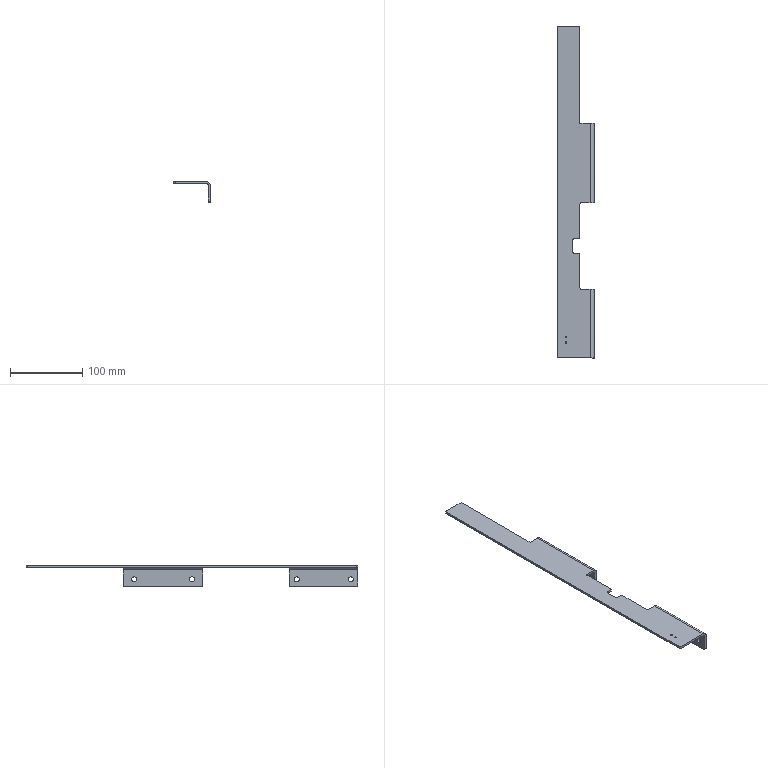Part | NX | features 5003_234_Bracket 2 | 1 solid | 39 faces | box 51 x 460 x 29 mm | volume 68788 mm3 | plane 20 | cylinder 19 | commonest cylinder face diameters 4 x9 7 x4 2.5 x2 6 x2 12 x2
STEP:
#1=CARTESIAN_POINT('',(-224.475,-262.,-64.));
#2=VERTEX_POINT('',#1);
#3=CARTESIAN_POINT('',(-227.475,-262.,-61.));
#4=VERTEX_POINT('',#3);
#5=CARTESIAN_POINT('',(-227.475,-262.,-64.));
#6=DIRECTION('',(0.,1.,0.));
#7=DIRECTION('',(-1.,0.,0.));
#8=AXIS2_PLACEMENT_3D('',#5,#6,#7);
#9=CIRCLE('',#8,3.);
#10=EDGE_CURVE('',#2,#4,#9,.F.);
#11=ORIENTED_EDGE('',*,*,#10,.T.);
#12=CARTESIAN_POINT('',(-227.475,-152.,-61.));
#13=VERTEX_POINT('',#12);
#14=CARTESIAN_POINT('',(-227.475,-477.,-61.));
#15=DIRECTION('',(0.,1.,0.));
#16=VECTOR('',#15,1000.);
#17=LINE('',#14,#16);
#18=EDGE_CURVE('',#4,#13,#17,.T.);
#19=ORIENTED_EDGE('',*,*,#18,.T.);
#20=CARTESIAN_POINT('',(-224.475,-152.,-64.));
#21=VERTEX_POINT('',#20);
#22=CARTESIAN_POINT('',(-227.475,-152.,-64.));
#23=DIRECTION('',(0.,-1.,0.));
#24=DIRECTION('',(1.,0.,0.));
#25=AXIS2_PLACEMENT_3D('',#22,#23,#24);
#26=CIRCLE('',#25,3.);
#27=EDGE_CURVE('',#13,#21,#26,.F.);
#28=ORIENTED_EDGE('',*,*,#27,.T.);
#29=CARTESIAN_POINT('',(-224.475,-477.,-64.));
#30=DIRECTION('',(0.,1.,0.));
#31=VECTOR('',#30,1000.);
#32=LINE('',#29,#31);
#33=EDGE_CURVE('',#2,#21,#32,.T.);
#34=ORIENTED_EDGE('',*,*,#33,.F.);
#35=EDGE_LOOP('',(#11,#19,#28,#34));
#36=FACE_BOUND('',#35,.T.);
#37=CARTESIAN_POINT('',(-227.475,-477.,-64.));
#38=DIRECTION('',(0.,1.,0.));
#39=DIRECTION('',(-1.,0.,0.));
#40=AXIS2_PLACEMENT_3D('',#37,#38,#39);
#41=CYLINDRICAL_SURFACE('',#40,3.);
#42=ADVANCED_FACE('',(#36),#41,.F.);
#43=CARTESIAN_POINT('',(-224.475,-262.,-87.));
#44=VERTEX_POINT('',#43);
#45=CARTESIAN_POINT('',(-224.475,-262.,-57.999));
#46=DIRECTION('',(0.,0.,1.));
#47=VECTOR('',#46,1000.);
#48=LINE('',#45,#47);
#49=EDGE_CURVE('',#44,#2,#48,.T.);
#50=ORIENTED_EDGE('',*,*,#49,.T.);
#51=ORIENTED_EDGE('',*,*,#33,.T.);
#52=CARTESIAN_POINT('',(-224.475,-152.,-87.));
#53=VERTEX_POINT('',#52);
#54=CARTESIAN_POINT('',(-224.475,-152.,-57.999));
#55=DIRECTION('',(0.,0.,-1.));
#56=VECTOR('',#55,1000.);
#57=LINE('',#54,#56);
#58=EDGE_CURVE('',#21,#53,#57,.T.);
#59=ORIENTED_EDGE('',*,*,#58,.T.);
#60=CARTESIAN_POINT('',(-224.475,-477.,-87.));
#61=DIRECTION('',(0.,1.,0.));
#62=VECTOR('',#61,1000.);
#63=LINE('',#60,#62);
#64=EDGE_CURVE('',#44,#53,#63,.T.);
#65=ORIENTED_EDGE('',*,*,#64,.F.);
#66=EDGE_LOOP('',(#50,#51,#59,#65));
#67=FACE_BOUND('',#66,.T.);
#68=CARTESIAN_POINT('',(-224.475,-247.,-73.5));
#69=VERTEX_POINT('',#68);
#70=CARTESIAN_POINT('',(-224.475,-247.,-77.));
#71=DIRECTION('',(-1.,0.,0.));
#72=DIRECTION('',(0.,0.,1.));
#73=AXIS2_PLACEMENT_3D('',#70,#71,#72);
#74=CIRCLE('',#73,3.5);
#75=EDGE_CURVE('',#69,#69,#74,.T.);
#76=ORIENTED_EDGE('',*,*,#75,.F.);
#77=EDGE_LOOP('',(#76));
#78=FACE_BOUND('',#77,.T.);
#79=CARTESIAN_POINT('',(-224.475,-167.,-73.5));
#80=VERTEX_POINT('',#79);
#81=CARTESIAN_POINT('',(-224.475,-167.,-77.));
#82=DIRECTION('',(-1.,0.,0.));
#83=DIRECTION('',(0.,0.,1.));
#84=AXIS2_PLACEMENT_3D('',#81,#82,#83);
#85=CIRCLE('',#84,3.5);
#86=EDGE_CURVE('',#80,#80,#85,.T.);
#87=ORIENTED_EDGE('',*,*,#86,.F.);
#88=EDGE_LOOP('',(#87));
#89=FACE_BOUND('',#88,.T.);
#90=CARTESIAN_POINT('',(-224.475,-477.,-87.));
#91=DIRECTION('',(-1.,0.,0.));
#92=DIRECTION('',(0.,0.,1.));
#93=AXIS2_PLACEMENT_3D('',#90,#91,#92);
#94=PLANE('',#93);
#95=ADVANCED_FACE('',(#67,#78,#89),#94,.T.);
#96=CARTESIAN_POINT('',(-221.475,-262.,-87.));
#97=VERTEX_POINT('',#96);
#98=CARTESIAN_POINT('',(-221.475,-262.,-87.));
#99=DIRECTION('',(1.,0.,0.));
#100=VECTOR('',#99,1000.);
#101=LINE('',#98,#100);
#102=EDGE_CURVE('',#44,#97,#101,.T.);
#103=ORIENTED_EDGE('',*,*,#102,.F.);
#104=ORIENTED_EDGE('',*,*,#64,.T.);
#105=CARTESIAN_POINT('',(-221.475,-152.,-87.));
#106=VERTEX_POINT('',#105);
#107=CARTESIAN_POINT('',(-221.475,-152.,-87.));
#108=DIRECTION('',(-1.,0.,0.));
#109=VECTOR('',#108,1000.);
#110=LINE('',#107,#109);
#111=EDGE_CURVE('',#106,#53,#110,.T.);
#112=ORIENTED_EDGE('',*,*,#111,.F.);
#113=CARTESIAN_POINT('',(-221.475,-477.,-87.));
#114=DIRECTION('',(0.,1.,0.));
#115=VECTOR('',#114,1000.);
#116=LINE('',#113,#115);
#117=EDGE_CURVE('',#97,#106,#116,.T.);
#118=ORIENTED_EDGE('',*,*,#117,.F.);
#119=EDGE_LOOP('',(#103,#104,#112,#118));
#120=FACE_BOUND('',#119,.T.);
#121=CARTESIAN_POINT('',(-221.475,-477.,-87.));
#122=DIRECTION('',(0.,0.,-1.));
#123=DIRECTION('',(0.,-1.,0.));
#124=AXIS2_PLACEMENT_3D('',#121,#122,#123);
#125=PLANE('',#124);
#126=ADVANCED_FACE('',(#120),#125,.T.);
#127=CARTESIAN_POINT('',(-221.475,-262.,-64.));
#128=VERTEX_POINT('',#127);
#129=CARTESIAN_POINT('',(-221.475,-262.,-57.999));
#130=DIRECTION('',(0.,0.,-1.));
#131=VECTOR('',#130,1000.);
#132=LINE('',#129,#131);
#133=EDGE_CURVE('',#128,#97,#132,.T.);
#134=ORIENTED_EDGE('',*,*,#133,.T.);
#135=ORIENTED_EDGE('',*,*,#117,.T.);
#136=CARTESIAN_POINT('',(-221.475,-152.,-64.));
#137=VERTEX_POINT('',#136);
#138=CARTESIAN_POINT('',(-221.475,-152.,-57.999));
#139=DIRECTION('',(0.,0.,-1.));
#140=VECTOR('',#139,1000.);
#141=LINE('',#138,#140);
#142=EDGE_CURVE('',#137,#106,#141,.T.);
#143=ORIENTED_EDGE('',*,*,#142,.F.);
#144=CARTESIAN_POINT('',(-221.475,-477.,-64.));
#145=DIRECTION('',(0.,1.,0.));
#146=VECTOR('',#145,1000.);
#147=LINE('',#144,#146);
#148=EDGE_CURVE('',#128,#137,#147,.T.);
#149=ORIENTED_EDGE('',*,*,#148,.F.);
#150=EDGE_LOOP('',(#134,#135,#143,#149));
#151=FACE_BOUND('',#150,.T.);
#152=CARTESIAN_POINT('',(-221.475,-247.,-73.5));
#153=VERTEX_POINT('',#152);
#154=CARTESIAN_POINT('',(-221.475,-247.,-77.));
#155=DIRECTION('',(-1.,0.,0.));
#156=DIRECTION('',(0.,0.,1.));
#157=AXIS2_PLACEMENT_3D('',#154,#155,#156);
#158=CIRCLE('',#157,3.5);
#159=EDGE_CURVE('',#153,#153,#158,.T.);
#160=ORIENTED_EDGE('',*,*,#159,.T.);
#161=EDGE_LOOP('',(#160));
#162=FACE_BOUND('',#161,.T.);
#163=CARTESIAN_POINT('',(-221.475,-167.,-73.5));
#164=VERTEX_POINT('',#163);
#165=CARTESIAN_POINT('',(-221.475,-167.,-77.));
#166=DIRECTION('',(-1.,0.,0.));
#167=DIRECTION('',(0.,0.,1.));
#168=AXIS2_PLACEMENT_3D('',#165,#166,#167);
#169=CIRCLE('',#168,3.5);
#170=EDGE_CURVE('',#164,#164,#169,.T.);
#171=ORIENTED_EDGE('',*,*,#170,.T.);
#172=EDGE_LOOP('',(#171));
#173=FACE_BOUND('',#172,.T.);
#174=CARTESIAN_POINT('',(-221.475,-477.,-64.));
#175=DIRECTION('',(1.,0.,0.));
#176=DIRECTION('',(0.,0.,-1.));
#177=AXIS2_PLACEMENT_3D('',#174,#175,#176);
#178=PLANE('',#177);
#179=ADVANCED_FACE('',(#151,#162,#173),#178,.T.);
#180=CARTESIAN_POINT('',(-227.475,-262.,-58.));
#181=VERTEX_POINT('',#180);
#182=CARTESIAN_POINT('',(-227.475,-262.,-64.));
#183=DIRECTION('',(0.,1.,0.));
#184=DIRECTION('',(-1.,0.,0.));
#185=AXIS2_PLACEMENT_3D('',#182,#183,#184);
#186=CIRCLE('',#185,6.);
#187=EDGE_CURVE('',#181,#128,#186,.T.);
#188=ORIENTED_EDGE('',*,*,#187,.T.);
#189=ORIENTED_EDGE('',*,*,#148,.T.);
#190=CARTESIAN_POINT('',(-227.475,-152.,-58.));
#191=VERTEX_POINT('',#190);
#192=CARTESIAN_POINT('',(-227.475,-152.,-64.));
#193=DIRECTION('',(0.,-1.,0.));
#194=DIRECTION('',(1.,0.,0.));
#195=AXIS2_PLACEMENT_3D('',#192,#193,#194);
#196=CIRCLE('',#195,6.);
#197=EDGE_CURVE('',#137,#191,#196,.T.);
#198=ORIENTED_EDGE('',*,*,#197,.T.);
#199=CARTESIAN_POINT('',(-227.475,-477.,-58.));
#200=DIRECTION('',(0.,1.,0.));
#201=VECTOR('',#200,1000.);
#202=LINE('',#199,#201);
#203=EDGE_CURVE('',#181,#191,#202,.T.);
#204=ORIENTED_EDGE('',*,*,#203,.F.);
#205=EDGE_LOOP('',(#188,#189,#198,#204));
#206=FACE_BOUND('',#205,.T.);
#207=CARTESIAN_POINT('',(-227.475,-477.,-64.));
#208=DIRECTION('',(0.,1.,0.));
#209=DIRECTION('',(-1.,0.,0.));
#210=AXIS2_PLACEMENT_3D('',#207,#208,#209);
#211=CYLINDRICAL_SURFACE('',#210,6.);
#212=ADVANCED_FACE('',(#206),#211,.T.);
#213=CARTESIAN_POINT('',(-272.475,-475.,-61.));
#214=VERTEX_POINT('',#213);
#215=CARTESIAN_POINT('',(-272.475,-19.,-61.));
#216=VERTEX_POINT('',#215);
#217=CARTESIAN_POINT('',(-272.475,-477.,-61.));
#218=DIRECTION('',(0.,1.,0.));
#219=VECTOR('',#218,1000.);
#220=LINE('',#217,#219);
#221=EDGE_CURVE('',#214,#216,#220,.T.);
#222=ORIENTED_EDGE('',*,*,#221,.F.);
#223=CARTESIAN_POINT('',(-272.475,-475.,-58.));
#224=VERTEX_POINT('',#223);
#225=CARTESIAN_POINT('',(-272.475,-475.,-58.));
#226=DIRECTION('',(0.,0.,1.));
#227=VECTOR('',#226,1000.);
#228=LINE('',#225,#227);
#229=EDGE_CURVE('',#214,#224,#228,.T.);
#230=ORIENTED_EDGE('',*,*,#229,.T.);
#231=CARTESIAN_POINT('',(-272.475,-19.,-58.));
#232=VERTEX_POINT('',#231);
#233=CARTESIAN_POINT('',(-272.475,-477.,-58.));
#234=DIRECTION('',(0.,1.,0.));
#235=VECTOR('',#234,1000.);
#236=LINE('',#233,#235);
#237=EDGE_CURVE('',#224,#232,#236,.T.);
#238=ORIENTED_EDGE('',*,*,#237,.T.);
#239=CARTESIAN_POINT('',(-272.475,-19.,-61.));
#240=DIRECTION('',(0.,0.,1.));
#241=VECTOR('',#240,1000.);
#242=LINE('',#239,#241);
#243=EDGE_CURVE('',#232,#216,#242,.F.);
#244=ORIENTED_EDGE('',*,*,#243,.T.);
#245=EDGE_LOOP('',(#222,#230,#238,#244));
#246=FACE_BOUND('',#245,.T.);
#247=CARTESIAN_POINT('',(-272.475,-477.,-58.));
#248=DIRECTION('',(-1.,0.,0.));
#249=DIRECTION('',(0.,-1.,0.));
#250=AXIS2_PLACEMENT_3D('',#247,#248,#249);
#251=PLANE('',#250);
#252=ADVANCED_FACE('',(#246),#251,.T.);
#253=CARTESIAN_POINT('',(-260.775,-449.29,-61.));
#254=VERTEX_POINT('',#253);
#255=CARTESIAN_POINT('',(-260.775,-448.04,-61.));
#256=DIRECTION('',(0.,0.,-1.));
#257=DIRECTION('',(0.,-1.,0.));
#258=AXIS2_PLACEMENT_3D('',#255,#256,#257);
#259=CIRCLE('',#258,1.25);
#260=EDGE_CURVE('',#254,#254,#259,.T.);
#261=ORIENTED_EDGE('',*,*,#260,.F.);
#262=EDGE_LOOP('',(#261));
#263=FACE_BOUND('',#262,.T.);
#264=CARTESIAN_POINT('',(-260.775,-457.29,-61.));
#265=VERTEX_POINT('',#264);
#266=CARTESIAN_POINT('',(-260.775,-456.04,-61.));
#267=DIRECTION('',(0.,0.,-1.));
#268=DIRECTION('',(0.,-1.,0.));
#269=AXIS2_PLACEMENT_3D('',#266,#267,#268);
#270=CIRCLE('',#269,1.25);
#271=EDGE_CURVE('',#265,#265,#270,.T.);
#272=ORIENTED_EDGE('',*,*,#271,.F.);
#273=EDGE_LOOP('',(#272));
#274=FACE_BOUND('',#273,.T.);
#275=CARTESIAN_POINT('',(-241.475,-264.,-61.));
#276=VERTEX_POINT('',#275);
#277=CARTESIAN_POINT('',(-241.475,-310.,-61.));
#278=VERTEX_POINT('',#277);
#279=CARTESIAN_POINT('',(-241.475,-262.,-61.));
#280=DIRECTION('',(0.,-1.,0.));
#281=VECTOR('',#280,1000.);
#282=LINE('',#279,#281);
#283=EDGE_CURVE('',#276,#278,#282,.T.);
#284=ORIENTED_EDGE('',*,*,#283,.T.);
#285=CARTESIAN_POINT('',(-243.475,-312.,-61.));
#286=VERTEX_POINT('',#285);
#287=CARTESIAN_POINT('',(-243.475,-310.,-61.));
#288=DIRECTION('',(0.,0.,-1.));
#289=DIRECTION('',(0.,-1.,0.));
#290=AXIS2_PLACEMENT_3D('',#287,#288,#289);
#291=CIRCLE('',#290,2.);
#292=EDGE_CURVE('',#278,#286,#291,.T.);
#293=ORIENTED_EDGE('',*,*,#292,.T.);
#294=CARTESIAN_POINT('',(-249.475,-312.,-61.));
#295=VERTEX_POINT('',#294);
#296=CARTESIAN_POINT('',(-241.475,-312.,-61.));
#297=DIRECTION('',(-1.,0.,0.));
#298=VECTOR('',#297,1000.);
#299=LINE('',#296,#298);
#300=EDGE_CURVE('',#286,#295,#299,.T.);
#301=ORIENTED_EDGE('',*,*,#300,.T.);
#302=CARTESIAN_POINT('',(-251.475,-314.,-61.));
#303=VERTEX_POINT('',#302);
#304=CARTESIAN_POINT('',(-249.475,-314.,-61.));
#305=DIRECTION('',(0.,0.,-1.));
#306=DIRECTION('',(0.,-1.,0.));
#307=AXIS2_PLACEMENT_3D('',#304,#305,#306);
#308=CIRCLE('',#307,2.);
#309=EDGE_CURVE('',#295,#303,#308,.F.);
#310=ORIENTED_EDGE('',*,*,#309,.T.);
#311=CARTESIAN_POINT('',(-251.475,-330.,-61.));
#312=VERTEX_POINT('',#311);
#313=CARTESIAN_POINT('',(-251.475,-312.,-61.));
#314=DIRECTION('',(0.,-1.,0.));
#315=VECTOR('',#314,1000.);
#316=LINE('',#313,#315);
#317=EDGE_CURVE('',#303,#312,#316,.T.);
#318=ORIENTED_EDGE('',*,*,#317,.T.);
#319=CARTESIAN_POINT('',(-249.475,-332.,-61.));
#320=VERTEX_POINT('',#319);
#321=CARTESIAN_POINT('',(-249.475,-330.,-61.));
#322=DIRECTION('',(0.,0.,-1.));
#323=DIRECTION('',(0.,-1.,0.));
#324=AXIS2_PLACEMENT_3D('',#321,#322,#323);
#325=CIRCLE('',#324,2.);
#326=EDGE_CURVE('',#312,#320,#325,.F.);
#327=ORIENTED_EDGE('',*,*,#326,.T.);
#328=CARTESIAN_POINT('',(-243.475,-332.,-61.));
#329=VERTEX_POINT('',#328);
#330=CARTESIAN_POINT('',(-251.475,-332.,-61.));
#331=DIRECTION('',(1.,0.,0.));
#332=VECTOR('',#331,1000.);
#333=LINE('',#330,#332);
#334=EDGE_CURVE('',#320,#329,#333,.T.);
#335=ORIENTED_EDGE('',*,*,#334,.T.);
#336=CARTESIAN_POINT('',(-241.475,-334.,-61.));
#337=VERTEX_POINT('',#336);
#338=CARTESIAN_POINT('',(-243.475,-334.,-61.));
#339=DIRECTION('',(0.,0.,-1.));
#340=DIRECTION('',(0.,-1.,0.));
#341=AXIS2_PLACEMENT_3D('',#338,#339,#340);
#342=CIRCLE('',#341,2.);
#343=EDGE_CURVE('',#329,#337,#342,.T.);
#344=ORIENTED_EDGE('',*,*,#343,.T.);
#345=CARTESIAN_POINT('',(-241.475,-380.,-61.));
#346=VERTEX_POINT('',#345);
#347=CARTESIAN_POINT('',(-241.475,-332.,-61.));
#348=DIRECTION('',(0.,-1.,0.));
#349=VECTOR('',#348,1000.);
#350=LINE('',#347,#349);
#351=EDGE_CURVE('',#337,#346,#350,.T.);
#352=ORIENTED_EDGE('',*,*,#351,.T.);
#353=CARTESIAN_POINT('',(-239.475,-382.,-61.));
#354=VERTEX_POINT('',#353);
#355=CARTESIAN_POINT('',(-239.475,-380.,-61.));
#356=DIRECTION('',(0.,0.,-1.));
#357=DIRECTION('',(0.,-1.,0.));
#358=AXIS2_PLACEMENT_3D('',#355,#356,#357);
#359=CIRCLE('',#358,2.);
#360=EDGE_CURVE('',#346,#354,#359,.F.);
#361=ORIENTED_EDGE('',*,*,#360,.T.);
#362=CARTESIAN_POINT('',(-227.475,-382.,-61.));
#363=VERTEX_POINT('',#362);
#364=CARTESIAN_POINT('',(-221.475,-382.,-61.));
#365=DIRECTION('',(1.,0.,0.));
#366=VECTOR('',#365,1000.);
#367=LINE('',#364,#366);
#368=EDGE_CURVE('',#354,#363,#367,.T.);
#369=ORIENTED_EDGE('',*,*,#368,.T.);
#370=CARTESIAN_POINT('',(-227.475,-477.,-61.));
#371=VERTEX_POINT('',#370);
#372=CARTESIAN_POINT('',(-227.475,-477.,-61.));
#373=DIRECTION('',(0.,1.,0.));
#374=VECTOR('',#373,1000.);
#375=LINE('',#372,#374);
#376=EDGE_CURVE('',#371,#363,#375,.T.);
#377=ORIENTED_EDGE('',*,*,#376,.F.);
#378=CARTESIAN_POINT('',(-270.475,-477.,-61.));
#379=VERTEX_POINT('',#378);
#380=CARTESIAN_POINT('',(-227.475,-477.,-61.));
#381=DIRECTION('',(-1.,0.,0.));
#382=VECTOR('',#381,1000.);
#383=LINE('',#380,#382);
#384=EDGE_CURVE('',#371,#379,#383,.T.);
#385=ORIENTED_EDGE('',*,*,#384,.T.);
#386=CARTESIAN_POINT('',(-270.475,-475.,-61.));
#387=DIRECTION('',(0.,0.,-1.));
#388=DIRECTION('',(0.,-1.,0.));
#389=AXIS2_PLACEMENT_3D('',#386,#387,#388);
#390=CIRCLE('',#389,2.);
#391=EDGE_CURVE('',#379,#214,#390,.T.);
#392=ORIENTED_EDGE('',*,*,#391,.T.);
#393=ORIENTED_EDGE('',*,*,#221,.T.);
#394=CARTESIAN_POINT('',(-270.475,-17.,-61.));
#395=VERTEX_POINT('',#394);
#396=CARTESIAN_POINT('',(-270.475,-19.,-61.));
#397=DIRECTION('',(0.,0.,-1.));
#398=DIRECTION('',(0.,-1.,0.));
#399=AXIS2_PLACEMENT_3D('',#396,#397,#398);
#400=CIRCLE('',#399,2.);
#401=EDGE_CURVE('',#216,#395,#400,.T.);
#402=ORIENTED_EDGE('',*,*,#401,.T.);
#403=CARTESIAN_POINT('',(-241.475,-17.,-61.));
#404=VERTEX_POINT('',#403);
#405=CARTESIAN_POINT('',(-227.475,-17.,-61.));
#406=DIRECTION('',(-1.,0.,0.));
#407=VECTOR('',#406,1000.);
#408=LINE('',#405,#407);
#409=EDGE_CURVE('',#404,#395,#408,.T.);
#410=ORIENTED_EDGE('',*,*,#409,.F.);
#411=CARTESIAN_POINT('',(-241.475,-152.,-61.));
#412=VERTEX_POINT('',#411);
#413=CARTESIAN_POINT('',(-241.475,-17.,-61.));
#414=DIRECTION('',(0.,-1.,0.));
#415=VECTOR('',#414,1000.);
#416=LINE('',#413,#415);
#417=EDGE_CURVE('',#404,#412,#416,.T.);
#418=ORIENTED_EDGE('',*,*,#417,.T.);
#419=CARTESIAN_POINT('',(-221.475,-152.,-61.));
#420=DIRECTION('',(1.,0.,0.));
#421=VECTOR('',#420,1000.);
#422=LINE('',#419,#421);
#423=EDGE_CURVE('',#412,#13,#422,.T.);
#424=ORIENTED_EDGE('',*,*,#423,.T.);
#425=ORIENTED_EDGE('',*,*,#18,.F.);
#426=CARTESIAN_POINT('',(-239.475,-262.,-61.));
#427=VERTEX_POINT('',#426);
#428=CARTESIAN_POINT('',(-221.475,-262.,-61.));
#429=DIRECTION('',(-1.,0.,0.));
#430=VECTOR('',#429,1000.);
#431=LINE('',#428,#430);
#432=EDGE_CURVE('',#4,#427,#431,.T.);
#433=ORIENTED_EDGE('',*,*,#432,.T.);
#434=CARTESIAN_POINT('',(-239.475,-264.,-61.));
#435=DIRECTION('',(0.,0.,-1.));
#436=DIRECTION('',(0.,-1.,0.));
#437=AXIS2_PLACEMENT_3D('',#434,#435,#436);
#438=CIRCLE('',#437,2.);
#439=EDGE_CURVE('',#427,#276,#438,.F.);
#440=ORIENTED_EDGE('',*,*,#439,.T.);
#441=EDGE_LOOP('',(#284,#293,#301,#310,#318,#327,#335,#344,#352,#361,#369,#377,#385,#392,#393,#402,#410,#418,#424,#425,#433,#440));
#442=FACE_BOUND('',#441,.T.);
#443=CARTESIAN_POINT('',(-227.475,-477.,-61.));
#444=DIRECTION('',(0.,0.,-1.));
#445=DIRECTION('',(0.,-1.,0.));
#446=AXIS2_PLACEMENT_3D('',#443,#444,#445);
#447=PLANE('',#446);
#448=ADVANCED_FACE('',(#263,#274,#442),#447,.T.);
#449=CARTESIAN_POINT('',(-224.475,-382.,-64.));
#450=VERTEX_POINT('',#449);
#451=CARTESIAN_POINT('',(-227.475,-382.,-64.));
#452=DIRECTION('',(0.,-1.,0.));
#453=DIRECTION('',(1.,0.,0.));
#454=AXIS2_PLACEMENT_3D('',#451,#452,#453);
#455=CIRCLE('',#454,3.);
#456=EDGE_CURVE('',#363,#450,#455,.F.);
#457=ORIENTED_EDGE('',*,*,#456,.T.);
#458=CARTESIAN_POINT('',(-224.475,-477.,-64.));
#459=VERTEX_POINT('',#458);
#460=CARTESIAN_POINT('',(-224.475,-477.,-64.));
#461=DIRECTION('',(0.,1.,0.));
#462=VECTOR('',#461,1000.);
#463=LINE('',#460,#462);
#464=EDGE_CURVE('',#459,#450,#463,.T.);
#465=ORIENTED_EDGE('',*,*,#464,.F.);
#466=CARTESIAN_POINT('',(-227.475,-477.,-64.));
#467=DIRECTION('',(0.,-1.,0.));
#468=DIRECTION('',(1.,0.,0.));
#469=AXIS2_PLACEMENT_3D('',#466,#467,#468);
#470=CIRCLE('',#469,3.);
#471=EDGE_CURVE('',#459,#371,#470,.T.);
#472=ORIENTED_EDGE('',*,*,#471,.T.);
#473=ORIENTED_EDGE('',*,*,#376,.T.);
#474=EDGE_LOOP('',(#457,#465,#472,#473));
#475=FACE_BOUND('',#474,.T.);
#476=CARTESIAN_POINT('',(-227.475,-477.,-64.));
#477=DIRECTION('',(0.,1.,0.));
#478=DIRECTION('',(-1.,0.,0.));
#479=AXIS2_PLACEMENT_3D('',#476,#477,#478);
#480=CYLINDRICAL_SURFACE('',#479,3.);
#481=ADVANCED_FACE('',(#475),#480,.F.);
#482=CARTESIAN_POINT('',(-224.475,-382.,-87.));
#483=VERTEX_POINT('',#482);
#484=CARTESIAN_POINT('',(-224.475,-382.,-57.999));
#485=DIRECTION('',(0.,0.,-1.));
#486=VECTOR('',#485,1000.);
#487=LINE('',#484,#486);
#488=EDGE_CURVE('',#450,#483,#487,.T.);
#489=ORIENTED_EDGE('',*,*,#488,.T.);
#490=CARTESIAN_POINT('',(-224.475,-475.,-87.));
#491=VERTEX_POINT('',#490);
#492=CARTESIAN_POINT('',(-224.475,-477.,-87.));
#493=DIRECTION('',(0.,1.,0.));
#494=VECTOR('',#493,1000.);
#495=LINE('',#492,#494);
#496=EDGE_CURVE('',#491,#483,#495,.T.);
#497=ORIENTED_EDGE('',*,*,#496,.F.);
#498=CARTESIAN_POINT('',(-224.475,-477.,-85.));
#499=VERTEX_POINT('',#498);
#500=CARTESIAN_POINT('',(-224.475,-475.,-85.));
#501=DIRECTION('',(-1.,0.,0.));
#502=DIRECTION('',(0.,0.,1.));
#503=AXIS2_PLACEMENT_3D('',#500,#501,#502);
#504=CIRCLE('',#503,2.);
#505=EDGE_CURVE('',#491,#499,#504,.T.);
#506=ORIENTED_EDGE('',*,*,#505,.T.);
#507=CARTESIAN_POINT('',(-224.475,-477.,-87.));
#508=DIRECTION('',(0.,0.,1.));
#509=VECTOR('',#508,1000.);
#510=LINE('',#507,#509);
#511=EDGE_CURVE('',#499,#459,#510,.T.);
#512=ORIENTED_EDGE('',*,*,#511,.T.);
#513=ORIENTED_EDGE('',*,*,#464,.T.);
#514=EDGE_LOOP('',(#489,#497,#506,#512,#513));
#515=FACE_BOUND('',#514,.T.);
#516=CARTESIAN_POINT('',(-224.475,-392.,-73.5));
#517=VERTEX_POINT('',#516);
#518=CARTESIAN_POINT('',(-224.475,-392.,-77.));
#519=DIRECTION('',(-1.,0.,0.));
#520=DIRECTION('',(0.,0.,1.));
#521=AXIS2_PLACEMENT_3D('',#518,#519,#520);
#522=CIRCLE('',#521,3.5);
#523=EDGE_CURVE('',#517,#517,#522,.T.);
#524=ORIENTED_EDGE('',*,*,#523,.F.);
#525=EDGE_LOOP('',(#524));
#526=FACE_BOUND('',#525,.T.);
#527=CARTESIAN_POINT('',(-224.475,-467.,-73.5));
#528=VERTEX_POINT('',#527);
#529=CARTESIAN_POINT('',(-224.475,-467.,-77.));
#530=DIRECTION('',(-1.,0.,0.));
#531=DIRECTION('',(0.,0.,1.));
#532=AXIS2_PLACEMENT_3D('',#529,#530,#531);
#533=CIRCLE('',#532,3.5);
#534=EDGE_CURVE('',#528,#528,#533,.T.);
#535=ORIENTED_EDGE('',*,*,#534,.F.);
#536=EDGE_LOOP('',(#535));
#537=FACE_BOUND('',#536,.T.);
#538=CARTESIAN_POINT('',(-224.475,-477.,-87.));
#539=DIRECTION('',(-1.,0.,0.));
#540=DIRECTION('',(0.,0.,1.));
#541=AXIS2_PLACEMENT_3D('',#538,#539,#540);
#542=PLANE('',#541);
#543=ADVANCED_FACE('',(#515,#526,#537),#542,.T.);
#544=CARTESIAN_POINT('',(-221.475,-382.,-87.));
#545=VERTEX_POINT('',#544);
#546=CARTESIAN_POINT('',(-221.475,-382.,-87.));
#547=DIRECTION('',(-1.,0.,0.));
#548=VECTOR('',#547,1000.);
#549=LINE('',#546,#548);
#550=EDGE_CURVE('',#545,#483,#549,.T.);
#551=ORIENTED_EDGE('',*,*,#550,.F.);
#552=CARTESIAN_POINT('',(-221.475,-475.,-87.));
#553=VERTEX_POINT('',#552);
#554=CARTESIAN_POINT('',(-221.475,-477.,-87.));
#555=DIRECTION('',(0.,1.,0.));
#556=VECTOR('',#555,1000.);
#557=LINE('',#554,#556);
#558=EDGE_CURVE('',#553,#545,#557,.T.);
#559=ORIENTED_EDGE('',*,*,#558,.F.);
#560=CARTESIAN_POINT('',(-221.475,-475.,-87.));
#561=DIRECTION('',(-1.,0.,0.));
#562=VECTOR('',#561,1000.);
#563=LINE('',#560,#562);
#564=EDGE_CURVE('',#553,#491,#563,.T.);
#565=ORIENTED_EDGE('',*,*,#564,.T.);
#566=ORIENTED_EDGE('',*,*,#496,.T.);
#567=EDGE_LOOP('',(#551,#559,#565,#566));
#568=FACE_BOUND('',#567,.T.);
#569=CARTESIAN_POINT('',(-221.475,-477.,-87.));
#570=DIRECTION('',(0.,0.,-1.));
#571=DIRECTION('',(0.,-1.,0.));
#572=AXIS2_PLACEMENT_3D('',#569,#570,#571);
#573=PLANE('',#572);
#574=ADVANCED_FACE('',(#568),#573,.T.);
#575=CARTESIAN_POINT('',(-221.475,-382.,-64.));
#576=VERTEX_POINT('',#575);
#577=CARTESIAN_POINT('',(-221.475,-382.,-57.999));
#578=DIRECTION('',(0.,0.,-1.));
#579=VECTOR('',#578,1000.);
#580=LINE('',#577,#579);
#581=EDGE_CURVE('',#576,#545,#580,.T.);
#582=ORIENTED_EDGE('',*,*,#581,.F.);
#583=CARTESIAN_POINT('',(-221.475,-477.,-64.));
#584=VERTEX_POINT('',#583);
#585=CARTESIAN_POINT('',(-221.475,-477.,-64.));
#586=DIRECTION('',(0.,1.,0.));
#587=VECTOR('',#586,1000.);
#588=LINE('',#585,#587);
#589=EDGE_CURVE('',#584,#576,#588,.T.);
#590=ORIENTED_EDGE('',*,*,#589,.F.);
#591=CARTESIAN_POINT('',(-221.475,-477.,-85.));
#592=VERTEX_POINT('',#591);
#593=CARTESIAN_POINT('',(-221.475,-477.,-64.));
#594=DIRECTION('',(0.,0.,-1.));
#595=VECTOR('',#594,1000.);
#596=LINE('',#593,#595);
#597=EDGE_CURVE('',#584,#592,#596,.T.);
#598=ORIENTED_EDGE('',*,*,#597,.T.);
#599=CARTESIAN_POINT('',(-221.475,-475.,-85.));
#600=DIRECTION('',(1.,0.,0.));
#601=DIRECTION('',(0.,0.,-1.));
#602=AXIS2_PLACEMENT_3D('',#599,#600,#601);
#603=CIRCLE('',#602,2.);
#604=EDGE_CURVE('',#592,#553,#603,.T.);
#605=ORIENTED_EDGE('',*,*,#604,.T.);
#606=ORIENTED_EDGE('',*,*,#558,.T.);
#607=EDGE_LOOP('',(#582,#590,#598,#605,#606));
#608=FACE_BOUND('',#607,.T.);
#609=CARTESIAN_POINT('',(-221.475,-392.,-73.5));
#610=VERTEX_POINT('',#609);
#611=CARTESIAN_POINT('',(-221.475,-392.,-77.));
#612=DIRECTION('',(-1.,0.,0.));
#613=DIRECTION('',(0.,0.,1.));
#614=AXIS2_PLACEMENT_3D('',#611,#612,#613);
#615=CIRCLE('',#614,3.5);
#616=EDGE_CURVE('',#610,#610,#615,.T.);
#617=ORIENTED_EDGE('',*,*,#616,.T.);
#618=EDGE_LOOP('',(#617));
#619=FACE_BOUND('',#618,.T.);
#620=CARTESIAN_POINT('',(-221.475,-467.,-73.5));
#621=VERTEX_POINT('',#620);
#622=CARTESIAN_POINT('',(-221.475,-467.,-77.));
#623=DIRECTION('',(-1.,0.,0.));
#624=DIRECTION('',(0.,0.,1.));
#625=AXIS2_PLACEMENT_3D('',#622,#623,#624);
#626=CIRCLE('',#625,3.5);
#627=EDGE_CURVE('',#621,#621,#626,.T.);
#628=ORIENTED_EDGE('',*,*,#627,.T.);
#629=EDGE_LOOP('',(#628));
#630=FACE_BOUND('',#629,.T.);
#631=CARTESIAN_POINT('',(-221.475,-477.,-64.));
#632=DIRECTION('',(1.,0.,0.));
#633=DIRECTION('',(0.,0.,-1.));
#634=AXIS2_PLACEMENT_3D('',#631,#632,#633);
#635=PLANE('',#634);
#636=ADVANCED_FACE('',(#608,#619,#630),#635,.T.);
#637=CARTESIAN_POINT('',(-227.475,-382.,-58.));
#638=VERTEX_POINT('',#637);
#639=CARTESIAN_POINT('',(-227.475,-382.,-64.));
#640=DIRECTION('',(0.,-1.,0.));
#641=DIRECTION('',(1.,0.,0.));
#642=AXIS2_PLACEMENT_3D('',#639,#640,#641);
#643=CIRCLE('',#642,6.);
#644=EDGE_CURVE('',#576,#638,#643,.T.);
#645=ORIENTED_EDGE('',*,*,#644,.T.);
#646=CARTESIAN_POINT('',(-227.475,-477.,-58.));
#647=VERTEX_POINT('',#646);
#648=CARTESIAN_POINT('',(-227.475,-477.,-58.));
#649=DIRECTION('',(0.,1.,0.));
#650=VECTOR('',#649,1000.);
#651=LINE('',#648,#650);
#652=EDGE_CURVE('',#647,#638,#651,.T.);
#653=ORIENTED_EDGE('',*,*,#652,.F.);
#654=CARTESIAN_POINT('',(-227.475,-477.,-64.));
#655=DIRECTION('',(0.,1.,0.));
#656=DIRECTION('',(1.,0.,0.));
#657=AXIS2_PLACEMENT_3D('',#654,#655,#656);
#658=CIRCLE('',#657,6.);
#659=EDGE_CURVE('',#647,#584,#658,.T.);
#660=ORIENTED_EDGE('',*,*,#659,.T.);
#661=ORIENTED_EDGE('',*,*,#589,.T.);
#662=EDGE_LOOP('',(#645,#653,#660,#661));
#663=FACE_BOUND('',#662,.T.);
#664=CARTESIAN_POINT('',(-227.475,-477.,-64.));
#665=DIRECTION('',(0.,1.,0.));
#666=DIRECTION('',(-1.,0.,0.));
#667=AXIS2_PLACEMENT_3D('',#664,#665,#666);
#668=CYLINDRICAL_SURFACE('',#667,6.);
#669=ADVANCED_FACE('',(#663),#668,.T.);
#670=CARTESIAN_POINT('',(-260.775,-446.79,-58.));
#671=VERTEX_POINT('',#670);
#672=CARTESIAN_POINT('',(-260.775,-448.04,-58.));
#673=DIRECTION('',(0.,0.,1.));
#674=DIRECTION('',(0.,1.,0.));
#675=AXIS2_PLACEMENT_3D('',#672,#673,#674);
#676=CIRCLE('',#675,1.25);
#677=EDGE_CURVE('',#671,#671,#676,.T.);
#678=ORIENTED_EDGE('',*,*,#677,.F.);
#679=EDGE_LOOP('',(#678));
#680=FACE_BOUND('',#679,.T.);
#681=CARTESIAN_POINT('',(-260.775,-454.79,-58.));
#682=VERTEX_POINT('',#681);
#683=CARTESIAN_POINT('',(-260.775,-456.04,-58.));
#684=DIRECTION('',(0.,0.,1.));
#685=DIRECTION('',(0.,1.,0.));
#686=AXIS2_PLACEMENT_3D('',#683,#684,#685);
#687=CIRCLE('',#686,1.25);
#688=EDGE_CURVE('',#682,#682,#687,.T.);
#689=ORIENTED_EDGE('',*,*,#688,.F.);
#690=EDGE_LOOP('',(#689));
#691=FACE_BOUND('',#690,.T.);
#692=CARTESIAN_POINT('',(-249.475,-312.,-58.));
#693=VERTEX_POINT('',#692);
#694=CARTESIAN_POINT('',(-243.475,-312.,-58.));
#695=VERTEX_POINT('',#694);
#696=CARTESIAN_POINT('',(-241.475,-312.,-58.));
#697=DIRECTION('',(1.,0.,0.));
#698=VECTOR('',#697,1000.);
#699=LINE('',#696,#698);
#700=EDGE_CURVE('',#693,#695,#699,.T.);
#701=ORIENTED_EDGE('',*,*,#700,.T.);
#702=CARTESIAN_POINT('',(-241.475,-310.,-58.));
#703=VERTEX_POINT('',#702);
#704=CARTESIAN_POINT('',(-243.475,-310.,-58.));
#705=DIRECTION('',(0.,0.,1.));
#706=DIRECTION('',(0.,1.,0.));
#707=AXIS2_PLACEMENT_3D('',#704,#705,#706);
#708=CIRCLE('',#707,2.);
#709=EDGE_CURVE('',#695,#703,#708,.T.);
#710=ORIENTED_EDGE('',*,*,#709,.T.);
#711=CARTESIAN_POINT('',(-241.475,-264.,-58.));
#712=VERTEX_POINT('',#711);
#713=CARTESIAN_POINT('',(-241.475,-262.,-58.));
#714=DIRECTION('',(0.,1.,0.));
#715=VECTOR('',#714,1000.);
#716=LINE('',#713,#715);
#717=EDGE_CURVE('',#703,#712,#716,.T.);
#718=ORIENTED_EDGE('',*,*,#717,.T.);
#719=CARTESIAN_POINT('',(-239.475,-262.,-58.));
#720=VERTEX_POINT('',#719);
#721=CARTESIAN_POINT('',(-239.475,-264.,-58.));
#722=DIRECTION('',(0.,0.,1.));
#723=DIRECTION('',(0.,1.,0.));
#724=AXIS2_PLACEMENT_3D('',#721,#722,#723);
#725=CIRCLE('',#724,2.);
#726=EDGE_CURVE('',#712,#720,#725,.F.);
#727=ORIENTED_EDGE('',*,*,#726,.T.);
#728=CARTESIAN_POINT('',(-221.475,-262.,-58.));
#729=DIRECTION('',(1.,0.,0.));
#730=VECTOR('',#729,1000.);
#731=LINE('',#728,#730);
#732=EDGE_CURVE('',#720,#181,#731,.T.);
#733=ORIENTED_EDGE('',*,*,#732,.T.);
#734=ORIENTED_EDGE('',*,*,#203,.T.);
#735=CARTESIAN_POINT('',(-241.475,-152.,-58.));
#736=VERTEX_POINT('',#735);
#737=CARTESIAN_POINT('',(-221.475,-152.,-58.));
#738=DIRECTION('',(-1.,0.,0.));
#739=VECTOR('',#738,1000.);
#740=LINE('',#737,#739);
#741=EDGE_CURVE('',#191,#736,#740,.T.);
#742=ORIENTED_EDGE('',*,*,#741,.T.);
#743=CARTESIAN_POINT('',(-241.475,-17.,-58.));
#744=VERTEX_POINT('',#743);
#745=CARTESIAN_POINT('',(-241.475,-17.,-58.));
#746=DIRECTION('',(0.,1.,0.));
#747=VECTOR('',#746,1000.);
#748=LINE('',#745,#747);
#749=EDGE_CURVE('',#736,#744,#748,.T.);
#750=ORIENTED_EDGE('',*,*,#749,.T.);
#751=CARTESIAN_POINT('',(-270.475,-17.,-58.));
#752=VERTEX_POINT('',#751);
#753=CARTESIAN_POINT('',(-227.475,-17.,-58.));
#754=DIRECTION('',(1.,0.,0.));
#755=VECTOR('',#754,1000.);
#756=LINE('',#753,#755);
#757=EDGE_CURVE('',#752,#744,#756,.T.);
#758=ORIENTED_EDGE('',*,*,#757,.F.);
#759=CARTESIAN_POINT('',(-270.475,-19.,-58.));
#760=DIRECTION('',(0.,0.,1.));
#761=DIRECTION('',(0.,1.,0.));
#762=AXIS2_PLACEMENT_3D('',#759,#760,#761);
#763=CIRCLE('',#762,2.);
#764=EDGE_CURVE('',#752,#232,#763,.T.);
#765=ORIENTED_EDGE('',*,*,#764,.T.);
#766=ORIENTED_EDGE('',*,*,#237,.F.);
#767=CARTESIAN_POINT('',(-270.475,-477.,-58.));
#768=VERTEX_POINT('',#767);
#769=CARTESIAN_POINT('',(-270.475,-475.,-58.));
#770=DIRECTION('',(0.,0.,1.));
#771=DIRECTION('',(0.,1.,0.));
#772=AXIS2_PLACEMENT_3D('',#769,#770,#771);
#773=CIRCLE('',#772,2.);
#774=EDGE_CURVE('',#224,#768,#773,.T.);
#775=ORIENTED_EDGE('',*,*,#774,.T.);
#776=CARTESIAN_POINT('',(-227.475,-477.,-58.));
#777=DIRECTION('',(1.,0.,0.));
#778=VECTOR('',#777,1000.);
#779=LINE('',#776,#778);
#780=EDGE_CURVE('',#768,#647,#779,.T.);
#781=ORIENTED_EDGE('',*,*,#780,.T.);
#782=ORIENTED_EDGE('',*,*,#652,.T.);
#783=CARTESIAN_POINT('',(-239.475,-382.,-58.));
#784=VERTEX_POINT('',#783);
#785=CARTESIAN_POINT('',(-221.475,-382.,-58.));
#786=DIRECTION('',(-1.,0.,0.));
#787=VECTOR('',#786,1000.);
#788=LINE('',#785,#787);
#789=EDGE_CURVE('',#638,#784,#788,.T.);
#790=ORIENTED_EDGE('',*,*,#789,.T.);
#791=CARTESIAN_POINT('',(-241.475,-380.,-58.));
#792=VERTEX_POINT('',#791);
#793=CARTESIAN_POINT('',(-239.475,-380.,-58.));
#794=DIRECTION('',(0.,0.,1.));
#795=DIRECTION('',(0.,1.,0.));
#796=AXIS2_PLACEMENT_3D('',#793,#794,#795);
#797=CIRCLE('',#796,2.);
#798=EDGE_CURVE('',#784,#792,#797,.F.);
#799=ORIENTED_EDGE('',*,*,#798,.T.);
#800=CARTESIAN_POINT('',(-241.475,-334.,-58.));
#801=VERTEX_POINT('',#800);
#802=CARTESIAN_POINT('',(-241.475,-332.,-58.));
#803=DIRECTION('',(0.,1.,0.));
#804=VECTOR('',#803,1000.);
#805=LINE('',#802,#804);
#806=EDGE_CURVE('',#792,#801,#805,.T.);
#807=ORIENTED_EDGE('',*,*,#806,.T.);
#808=CARTESIAN_POINT('',(-243.475,-332.,-58.));
#809=VERTEX_POINT('',#808);
#810=CARTESIAN_POINT('',(-243.475,-334.,-58.));
#811=DIRECTION('',(0.,0.,1.));
#812=DIRECTION('',(0.,1.,0.));
#813=AXIS2_PLACEMENT_3D('',#810,#811,#812);
#814=CIRCLE('',#813,2.);
#815=EDGE_CURVE('',#801,#809,#814,.T.);
#816=ORIENTED_EDGE('',*,*,#815,.T.);
#817=CARTESIAN_POINT('',(-249.475,-332.,-58.));
#818=VERTEX_POINT('',#817);
#819=CARTESIAN_POINT('',(-251.475,-332.,-58.));
#820=DIRECTION('',(-1.,0.,0.));
#821=VECTOR('',#820,1000.);
#822=LINE('',#819,#821);
#823=EDGE_CURVE('',#809,#818,#822,.T.);
#824=ORIENTED_EDGE('',*,*,#823,.T.);
#825=CARTESIAN_POINT('',(-251.475,-330.,-58.));
#826=VERTEX_POINT('',#825);
#827=CARTESIAN_POINT('',(-249.475,-330.,-58.));
#828=DIRECTION('',(0.,0.,1.));
#829=DIRECTION('',(0.,1.,0.));
#830=AXIS2_PLACEMENT_3D('',#827,#828,#829);
#831=CIRCLE('',#830,2.);
#832=EDGE_CURVE('',#818,#826,#831,.F.);
#833=ORIENTED_EDGE('',*,*,#832,.T.);
#834=CARTESIAN_POINT('',(-251.475,-314.,-58.));
#835=VERTEX_POINT('',#834);
#836=CARTESIAN_POINT('',(-251.475,-312.,-58.));
#837=DIRECTION('',(0.,1.,0.));
#838=VECTOR('',#837,1000.);
#839=LINE('',#836,#838);
#840=EDGE_CURVE('',#826,#835,#839,.T.);
#841=ORIENTED_EDGE('',*,*,#840,.T.);
#842=CARTESIAN_POINT('',(-249.475,-314.,-58.));
#843=DIRECTION('',(0.,0.,1.));
#844=DIRECTION('',(0.,1.,0.));
#845=AXIS2_PLACEMENT_3D('',#842,#843,#844);
#846=CIRCLE('',#845,2.);
#847=EDGE_CURVE('',#835,#693,#846,.F.);
#848=ORIENTED_EDGE('',*,*,#847,.T.);
#849=EDGE_LOOP('',(#701,#710,#718,#727,#733,#734,#742,#750,#758,#765,#766,#775,#781,#782,#790,#799,#807,#816,#824,#833,#841,#848));
#850=FACE_BOUND('',#849,.T.);
#851=CARTESIAN_POINT('',(-227.475,-477.,-58.));
#852=DIRECTION('',(0.,0.,1.));
#853=DIRECTION('',(0.,1.,0.));
#854=AXIS2_PLACEMENT_3D('',#851,#852,#853);
#855=PLANE('',#854);
#856=ADVANCED_FACE('',(#680,#691,#850),#855,.T.);
#857=ORIENTED_EDGE('',*,*,#511,.F.);
#858=CARTESIAN_POINT('',(-227.475,-477.,-85.));
#859=DIRECTION('',(-1.,0.,0.));
#860=VECTOR('',#859,1000.);
#861=LINE('',#858,#860);
#862=EDGE_CURVE('',#499,#592,#861,.F.);
#863=ORIENTED_EDGE('',*,*,#862,.T.);
#864=ORIENTED_EDGE('',*,*,#597,.F.);
#865=ORIENTED_EDGE('',*,*,#659,.F.);
#866=ORIENTED_EDGE('',*,*,#780,.F.);
#867=CARTESIAN_POINT('',(-270.475,-477.,-64.));
#868=DIRECTION('',(0.,0.,1.));
#869=VECTOR('',#868,1000.);
#870=LINE('',#867,#869);
#871=EDGE_CURVE('',#768,#379,#870,.F.);
#872=ORIENTED_EDGE('',*,*,#871,.T.);
#873=ORIENTED_EDGE('',*,*,#384,.F.);
#874=ORIENTED_EDGE('',*,*,#471,.F.);
#875=EDGE_LOOP('',(#857,#863,#864,#865,#866,#872,#873,#874));
#876=FACE_BOUND('',#875,.T.);
#877=CARTESIAN_POINT('',(-227.475,-477.,-64.));
#878=DIRECTION('',(0.,-1.,0.));
#879=DIRECTION('',(1.,0.,0.));
#880=AXIS2_PLACEMENT_3D('',#877,#878,#879);
#881=PLANE('',#880);
#882=ADVANCED_FACE('',(#876),#881,.T.);
#883=ORIENTED_EDGE('',*,*,#757,.T.);
#884=CARTESIAN_POINT('',(-241.475,-17.,-57.999));
#885=DIRECTION('',(0.,0.,-1.));
#886=VECTOR('',#885,1000.);
#887=LINE('',#884,#886);
#888=EDGE_CURVE('',#744,#404,#887,.T.);
#889=ORIENTED_EDGE('',*,*,#888,.T.);
#890=ORIENTED_EDGE('',*,*,#409,.T.);
#891=CARTESIAN_POINT('',(-270.475,-17.,-58.));
#892=DIRECTION('',(0.,0.,1.));
#893=VECTOR('',#892,1000.);
#894=LINE('',#891,#893);
#895=EDGE_CURVE('',#395,#752,#894,.T.);
#896=ORIENTED_EDGE('',*,*,#895,.T.);
#897=EDGE_LOOP('',(#883,#889,#890,#896));
#898=FACE_BOUND('',#897,.T.);
#899=CARTESIAN_POINT('',(-227.475,-17.,-64.));
#900=DIRECTION('',(0.,-1.,0.));
#901=DIRECTION('',(1.,0.,0.));
#902=AXIS2_PLACEMENT_3D('',#899,#900,#901);
#903=PLANE('',#902);
#904=ADVANCED_FACE('',(#898),#903,.F.);
#905=ORIENTED_EDGE('',*,*,#627,.F.);
#906=EDGE_LOOP('',(#905));
#907=FACE_BOUND('',#906,.T.);
#908=ORIENTED_EDGE('',*,*,#534,.T.);
#909=EDGE_LOOP('',(#908));
#910=FACE_BOUND('',#909,.T.);
#911=CARTESIAN_POINT('',(-221.475,-467.,-77.));
#912=DIRECTION('',(-1.,0.,0.));
#913=DIRECTION('',(0.,0.,1.));
#914=AXIS2_PLACEMENT_3D('',#911,#912,#913);
#915=CYLINDRICAL_SURFACE('',#914,3.5);
#916=ADVANCED_FACE('',(#907,#910),#915,.F.);
#917=ORIENTED_EDGE('',*,*,#616,.F.);
#918=EDGE_LOOP('',(#917));
#919=FACE_BOUND('',#918,.T.);
#920=ORIENTED_EDGE('',*,*,#523,.T.);
#921=EDGE_LOOP('',(#920));
#922=FACE_BOUND('',#921,.T.);
#923=CARTESIAN_POINT('',(-221.475,-392.,-77.));
#924=DIRECTION('',(-1.,0.,0.));
#925=DIRECTION('',(0.,0.,1.));
#926=AXIS2_PLACEMENT_3D('',#923,#924,#925);
#927=CYLINDRICAL_SURFACE('',#926,3.5);
#928=ADVANCED_FACE('',(#919,#922),#927,.F.);
#929=ORIENTED_EDGE('',*,*,#159,.F.);
#930=EDGE_LOOP('',(#929));
#931=FACE_BOUND('',#930,.T.);
#932=ORIENTED_EDGE('',*,*,#75,.T.);
#933=EDGE_LOOP('',(#932));
#934=FACE_BOUND('',#933,.T.);
#935=CARTESIAN_POINT('',(-221.475,-247.,-77.));
#936=DIRECTION('',(-1.,0.,0.));
#937=DIRECTION('',(0.,0.,1.));
#938=AXIS2_PLACEMENT_3D('',#935,#936,#937);
#939=CYLINDRICAL_SURFACE('',#938,3.5);
#940=ADVANCED_FACE('',(#931,#934),#939,.F.);
#941=ORIENTED_EDGE('',*,*,#170,.F.);
#942=EDGE_LOOP('',(#941));
#943=FACE_BOUND('',#942,.T.);
#944=ORIENTED_EDGE('',*,*,#86,.T.);
#945=EDGE_LOOP('',(#944));
#946=FACE_BOUND('',#945,.T.);
#947=CARTESIAN_POINT('',(-221.475,-167.,-77.));
#948=DIRECTION('',(-1.,0.,0.));
#949=DIRECTION('',(0.,0.,1.));
#950=AXIS2_PLACEMENT_3D('',#947,#948,#949);
#951=CYLINDRICAL_SURFACE('',#950,3.5);
#952=ADVANCED_FACE('',(#943,#946),#951,.F.);
#953=ORIENTED_EDGE('',*,*,#604,.F.);
#954=ORIENTED_EDGE('',*,*,#862,.F.);
#955=ORIENTED_EDGE('',*,*,#505,.F.);
#956=ORIENTED_EDGE('',*,*,#564,.F.);
#957=EDGE_LOOP('',(#953,#954,#955,#956));
#958=FACE_BOUND('',#957,.T.);
#959=CARTESIAN_POINT('',(-221.475,-475.,-85.));
#960=DIRECTION('',(-1.,0.,0.));
#961=DIRECTION('',(0.,-1.,0.));
#962=AXIS2_PLACEMENT_3D('',#959,#960,#961);
#963=CYLINDRICAL_SURFACE('',#962,2.);
#964=ADVANCED_FACE('',(#958),#963,.T.);
#965=ORIENTED_EDGE('',*,*,#391,.F.);
#966=ORIENTED_EDGE('',*,*,#871,.F.);
#967=ORIENTED_EDGE('',*,*,#774,.F.);
#968=ORIENTED_EDGE('',*,*,#229,.F.);
#969=EDGE_LOOP('',(#965,#966,#967,#968));
#970=FACE_BOUND('',#969,.T.);
#971=CARTESIAN_POINT('',(-270.475,-475.,-58.));
#972=DIRECTION('',(0.,0.,1.));
#973=DIRECTION('',(0.,1.,0.));
#974=AXIS2_PLACEMENT_3D('',#971,#972,#973);
#975=CYLINDRICAL_SURFACE('',#974,2.);
#976=ADVANCED_FACE('',(#970),#975,.T.);
#977=ORIENTED_EDGE('',*,*,#401,.F.);
#978=ORIENTED_EDGE('',*,*,#243,.F.);
#979=ORIENTED_EDGE('',*,*,#764,.F.);
#980=ORIENTED_EDGE('',*,*,#895,.F.);
#981=EDGE_LOOP('',(#977,#978,#979,#980));
#982=FACE_BOUND('',#981,.T.);
#983=CARTESIAN_POINT('',(-270.475,-19.,-64.));
#984=DIRECTION('',(0.,0.,-1.));
#985=DIRECTION('',(0.,-1.,0.));
#986=AXIS2_PLACEMENT_3D('',#983,#984,#985);
#987=CYLINDRICAL_SURFACE('',#986,2.);
#988=ADVANCED_FACE('',(#982),#987,.T.);
#989=ORIENTED_EDGE('',*,*,#888,.F.);
#990=ORIENTED_EDGE('',*,*,#749,.F.);
#991=CARTESIAN_POINT('',(-241.475,-152.,-57.999));
#992=DIRECTION('',(0.,0.,-1.));
#993=VECTOR('',#992,1000.);
#994=LINE('',#991,#993);
#995=EDGE_CURVE('',#736,#412,#994,.T.);
#996=ORIENTED_EDGE('',*,*,#995,.T.);
#997=ORIENTED_EDGE('',*,*,#417,.F.);
#998=EDGE_LOOP('',(#989,#990,#996,#997));
#999=FACE_BOUND('',#998,.T.);
#1000=CARTESIAN_POINT('',(-241.475,-17.,-57.999));
#1001=DIRECTION('',(-1.,0.,0.));
#1002=DIRECTION('',(0.,-1.,0.));
#1003=AXIS2_PLACEMENT_3D('',#1000,#1001,#1002);
#1004=PLANE('',#1003);
#1005=ADVANCED_FACE('',(#999),#1004,.F.);
#1006=ORIENTED_EDGE('',*,*,#995,.F.);
#1007=ORIENTED_EDGE('',*,*,#741,.F.);
#1008=ORIENTED_EDGE('',*,*,#197,.F.);
#1009=ORIENTED_EDGE('',*,*,#142,.T.);
#1010=ORIENTED_EDGE('',*,*,#111,.T.);
#1011=ORIENTED_EDGE('',*,*,#58,.F.);
#1012=ORIENTED_EDGE('',*,*,#27,.F.);
#1013=ORIENTED_EDGE('',*,*,#423,.F.);
#1014=EDGE_LOOP('',(#1006,#1007,#1008,#1009,#1010,#1011,#1012,#1013));
#1015=FACE_BOUND('',#1014,.T.);
#1016=CARTESIAN_POINT('',(-221.475,-152.,-57.999));
#1017=DIRECTION('',(0.,-1.,0.));
#1018=DIRECTION('',(1.,0.,0.));
#1019=AXIS2_PLACEMENT_3D('',#1016,#1017,#1018);
#1020=PLANE('',#1019);
#1021=ADVANCED_FACE('',(#1015),#1020,.F.);
#1022=ORIENTED_EDGE('',*,*,#732,.F.);
#1023=CARTESIAN_POINT('',(-239.475,-262.,-61.));
#1024=DIRECTION('',(0.,0.,-1.));
#1025=VECTOR('',#1024,1000.);
#1026=LINE('',#1023,#1025);
#1027=EDGE_CURVE('',#720,#427,#1026,.T.);
#1028=ORIENTED_EDGE('',*,*,#1027,.T.);
#1029=ORIENTED_EDGE('',*,*,#432,.F.);
#1030=ORIENTED_EDGE('',*,*,#10,.F.);
#1031=ORIENTED_EDGE('',*,*,#49,.F.);
#1032=ORIENTED_EDGE('',*,*,#102,.T.);
#1033=ORIENTED_EDGE('',*,*,#133,.F.);
#1034=ORIENTED_EDGE('',*,*,#187,.F.);
#1035=EDGE_LOOP('',(#1022,#1028,#1029,#1030,#1031,#1032,#1033,#1034));
#1036=FACE_BOUND('',#1035,.T.);
#1037=CARTESIAN_POINT('',(-221.475,-262.,-57.999));
#1038=DIRECTION('',(0.,1.,0.));
#1039=DIRECTION('',(-1.,0.,0.));
#1040=AXIS2_PLACEMENT_3D('',#1037,#1038,#1039);
#1041=PLANE('',#1040);
#1042=ADVANCED_FACE('',(#1036),#1041,.F.);
#1043=ORIENTED_EDGE('',*,*,#283,.F.);
#1044=CARTESIAN_POINT('',(-241.475,-264.,-58.));
#1045=DIRECTION('',(0.,0.,-1.));
#1046=VECTOR('',#1045,1000.);
#1047=LINE('',#1044,#1046);
#1048=EDGE_CURVE('',#276,#712,#1047,.F.);
#1049=ORIENTED_EDGE('',*,*,#1048,.T.);
#1050=ORIENTED_EDGE('',*,*,#717,.F.);
#1051=CARTESIAN_POINT('',(-241.475,-310.,-57.999));
#1052=DIRECTION('',(0.,0.,-1.));
#1053=VECTOR('',#1052,1000.);
#1054=LINE('',#1051,#1053);
#1055=EDGE_CURVE('',#703,#278,#1054,.T.);
#1056=ORIENTED_EDGE('',*,*,#1055,.T.);
#1057=EDGE_LOOP('',(#1043,#1049,#1050,#1056));
#1058=FACE_BOUND('',#1057,.T.);
#1059=CARTESIAN_POINT('',(-241.475,-262.,-57.999));
#1060=DIRECTION('',(-1.,0.,0.));
#1061=DIRECTION('',(0.,-1.,0.));
#1062=AXIS2_PLACEMENT_3D('',#1059,#1060,#1061);
#1063=PLANE('',#1062);
#1064=ADVANCED_FACE('',(#1058),#1063,.F.);
#1065=ORIENTED_EDGE('',*,*,#300,.F.);
#1066=CARTESIAN_POINT('',(-243.475,-312.,-57.999));
#1067=DIRECTION('',(0.,0.,-1.));
#1068=VECTOR('',#1067,1000.);
#1069=LINE('',#1066,#1068);
#1070=EDGE_CURVE('',#286,#695,#1069,.F.);
#1071=ORIENTED_EDGE('',*,*,#1070,.T.);
#1072=ORIENTED_EDGE('',*,*,#700,.F.);
#1073=CARTESIAN_POINT('',(-249.475,-312.,-61.));
#1074=DIRECTION('',(0.,0.,-1.));
#1075=VECTOR('',#1074,1000.);
#1076=LINE('',#1073,#1075);
#1077=EDGE_CURVE('',#693,#295,#1076,.T.);
#1078=ORIENTED_EDGE('',*,*,#1077,.T.);
#1079=EDGE_LOOP('',(#1065,#1071,#1072,#1078));
#1080=FACE_BOUND('',#1079,.T.);
#1081=CARTESIAN_POINT('',(-241.475,-312.,-57.999));
#1082=DIRECTION('',(0.,1.,0.));
#1083=DIRECTION('',(-1.,0.,0.));
#1084=AXIS2_PLACEMENT_3D('',#1081,#1082,#1083);
#1085=PLANE('',#1084);
#1086=ADVANCED_FACE('',(#1080),#1085,.F.);
#1087=ORIENTED_EDGE('',*,*,#317,.F.);
#1088=CARTESIAN_POINT('',(-251.475,-314.,-58.));
#1089=DIRECTION('',(0.,0.,-1.));
#1090=VECTOR('',#1089,1000.);
#1091=LINE('',#1088,#1090);
#1092=EDGE_CURVE('',#303,#835,#1091,.F.);
#1093=ORIENTED_EDGE('',*,*,#1092,.T.);
#1094=ORIENTED_EDGE('',*,*,#840,.F.);
#1095=CARTESIAN_POINT('',(-251.475,-330.,-61.));
#1096=DIRECTION('',(0.,0.,-1.));
#1097=VECTOR('',#1096,1000.);
#1098=LINE('',#1095,#1097);
#1099=EDGE_CURVE('',#826,#312,#1098,.T.);
#1100=ORIENTED_EDGE('',*,*,#1099,.T.);
#1101=EDGE_LOOP('',(#1087,#1093,#1094,#1100));
#1102=FACE_BOUND('',#1101,.T.);
#1103=CARTESIAN_POINT('',(-251.475,-312.,-57.999));
#1104=DIRECTION('',(-1.,0.,0.));
#1105=DIRECTION('',(0.,-1.,0.));
#1106=AXIS2_PLACEMENT_3D('',#1103,#1104,#1105);
#1107=PLANE('',#1106);
#1108=ADVANCED_FACE('',(#1102),#1107,.F.);
#1109=ORIENTED_EDGE('',*,*,#334,.F.);
#1110=CARTESIAN_POINT('',(-249.475,-332.,-58.));
#1111=DIRECTION('',(0.,0.,-1.));
#1112=VECTOR('',#1111,1000.);
#1113=LINE('',#1110,#1112);
#1114=EDGE_CURVE('',#320,#818,#1113,.F.);
#1115=ORIENTED_EDGE('',*,*,#1114,.T.);
#1116=ORIENTED_EDGE('',*,*,#823,.F.);
#1117=CARTESIAN_POINT('',(-243.475,-332.,-57.999));
#1118=DIRECTION('',(0.,0.,-1.));
#1119=VECTOR('',#1118,1000.);
#1120=LINE('',#1117,#1119);
#1121=EDGE_CURVE('',#809,#329,#1120,.T.);
#1122=ORIENTED_EDGE('',*,*,#1121,.T.);
#1123=EDGE_LOOP('',(#1109,#1115,#1116,#1122));
#1124=FACE_BOUND('',#1123,.T.);
#1125=CARTESIAN_POINT('',(-251.475,-332.,-57.999));
#1126=DIRECTION('',(0.,-1.,0.));
#1127=DIRECTION('',(1.,0.,0.));
#1128=AXIS2_PLACEMENT_3D('',#1125,#1126,#1127);
#1129=PLANE('',#1128);
#1130=ADVANCED_FACE('',(#1124),#1129,.F.);
#1131=ORIENTED_EDGE('',*,*,#351,.F.);
#1132=CARTESIAN_POINT('',(-241.475,-334.,-57.999));
#1133=DIRECTION('',(0.,0.,-1.));
#1134=VECTOR('',#1133,1000.);
#1135=LINE('',#1132,#1134);
#1136=EDGE_CURVE('',#337,#801,#1135,.F.);
#1137=ORIENTED_EDGE('',*,*,#1136,.T.);
#1138=ORIENTED_EDGE('',*,*,#806,.F.);
#1139=CARTESIAN_POINT('',(-241.475,-380.,-61.));
#1140=DIRECTION('',(0.,0.,-1.));
#1141=VECTOR('',#1140,1000.);
#1142=LINE('',#1139,#1141);
#1143=EDGE_CURVE('',#792,#346,#1142,.T.);
#1144=ORIENTED_EDGE('',*,*,#1143,.T.);
#1145=EDGE_LOOP('',(#1131,#1137,#1138,#1144));
#1146=FACE_BOUND('',#1145,.T.);
#1147=CARTESIAN_POINT('',(-241.475,-332.,-57.999));
#1148=DIRECTION('',(-1.,0.,0.));
#1149=DIRECTION('',(0.,-1.,0.));
#1150=AXIS2_PLACEMENT_3D('',#1147,#1148,#1149);
#1151=PLANE('',#1150);
#1152=ADVANCED_FACE('',(#1146),#1151,.F.);
#1153=ORIENTED_EDGE('',*,*,#368,.F.);
#1154=CARTESIAN_POINT('',(-239.475,-382.,-58.));
#1155=DIRECTION('',(0.,0.,-1.));
#1156=VECTOR('',#1155,1000.);
#1157=LINE('',#1154,#1156);
#1158=EDGE_CURVE('',#354,#784,#1157,.F.);
#1159=ORIENTED_EDGE('',*,*,#1158,.T.);
#1160=ORIENTED_EDGE('',*,*,#789,.F.);
#1161=ORIENTED_EDGE('',*,*,#644,.F.);
#1162=ORIENTED_EDGE('',*,*,#581,.T.);
#1163=ORIENTED_EDGE('',*,*,#550,.T.);
#1164=ORIENTED_EDGE('',*,*,#488,.F.);
#1165=ORIENTED_EDGE('',*,*,#456,.F.);
#1166=EDGE_LOOP('',(#1153,#1159,#1160,#1161,#1162,#1163,#1164,#1165));
#1167=FACE_BOUND('',#1166,.T.);
#1168=CARTESIAN_POINT('',(-221.475,-382.,-57.999));
#1169=DIRECTION('',(0.,-1.,0.));
#1170=DIRECTION('',(1.,0.,0.));
#1171=AXIS2_PLACEMENT_3D('',#1168,#1169,#1170);
#1172=PLANE('',#1171);
#1173=ADVANCED_FACE('',(#1167),#1172,.F.);
#1174=ORIENTED_EDGE('',*,*,#726,.F.);
#1175=ORIENTED_EDGE('',*,*,#1048,.F.);
#1176=ORIENTED_EDGE('',*,*,#439,.F.);
#1177=ORIENTED_EDGE('',*,*,#1027,.F.);
#1178=EDGE_LOOP('',(#1174,#1175,#1176,#1177));
#1179=FACE_BOUND('',#1178,.T.);
#1180=CARTESIAN_POINT('',(-239.475,-264.,-57.999));
#1181=DIRECTION('',(0.,0.,1.));
#1182=DIRECTION('',(0.,1.,0.));
#1183=AXIS2_PLACEMENT_3D('',#1180,#1181,#1182);
#1184=CYLINDRICAL_SURFACE('',#1183,2.);
#1185=ADVANCED_FACE('',(#1179),#1184,.F.);
#1186=ORIENTED_EDGE('',*,*,#709,.F.);
#1187=ORIENTED_EDGE('',*,*,#1070,.F.);
#1188=ORIENTED_EDGE('',*,*,#292,.F.);
#1189=ORIENTED_EDGE('',*,*,#1055,.F.);
#1190=EDGE_LOOP('',(#1186,#1187,#1188,#1189));
#1191=FACE_BOUND('',#1190,.T.);
#1192=CARTESIAN_POINT('',(-243.475,-310.,-57.999));
#1193=DIRECTION('',(0.,0.,-1.));
#1194=DIRECTION('',(0.,-1.,0.));
#1195=AXIS2_PLACEMENT_3D('',#1192,#1193,#1194);
#1196=CYLINDRICAL_SURFACE('',#1195,2.);
#1197=ADVANCED_FACE('',(#1191),#1196,.T.);
#1198=ORIENTED_EDGE('',*,*,#847,.F.);
#1199=ORIENTED_EDGE('',*,*,#1092,.F.);
#1200=ORIENTED_EDGE('',*,*,#309,.F.);
#1201=ORIENTED_EDGE('',*,*,#1077,.F.);
#1202=EDGE_LOOP('',(#1198,#1199,#1200,#1201));
#1203=FACE_BOUND('',#1202,.T.);
#1204=CARTESIAN_POINT('',(-249.475,-314.,-57.999));
#1205=DIRECTION('',(0.,0.,1.));
#1206=DIRECTION('',(0.,1.,0.));
#1207=AXIS2_PLACEMENT_3D('',#1204,#1205,#1206);
#1208=CYLINDRICAL_SURFACE('',#1207,2.);
#1209=ADVANCED_FACE('',(#1203),#1208,.F.);
#1210=ORIENTED_EDGE('',*,*,#832,.F.);
#1211=ORIENTED_EDGE('',*,*,#1114,.F.);
#1212=ORIENTED_EDGE('',*,*,#326,.F.);
#1213=ORIENTED_EDGE('',*,*,#1099,.F.);
#1214=EDGE_LOOP('',(#1210,#1211,#1212,#1213));
#1215=FACE_BOUND('',#1214,.T.);
#1216=CARTESIAN_POINT('',(-249.475,-330.,-57.999));
#1217=DIRECTION('',(0.,0.,1.));
#1218=DIRECTION('',(0.,1.,0.));
#1219=AXIS2_PLACEMENT_3D('',#1216,#1217,#1218);
#1220=CYLINDRICAL_SURFACE('',#1219,2.);
#1221=ADVANCED_FACE('',(#1215),#1220,.F.);
#1222=ORIENTED_EDGE('',*,*,#815,.F.);
#1223=ORIENTED_EDGE('',*,*,#1136,.F.);
#1224=ORIENTED_EDGE('',*,*,#343,.F.);
#1225=ORIENTED_EDGE('',*,*,#1121,.F.);
#1226=EDGE_LOOP('',(#1222,#1223,#1224,#1225));
#1227=FACE_BOUND('',#1226,.T.);
#1228=CARTESIAN_POINT('',(-243.475,-334.,-57.999));
#1229=DIRECTION('',(0.,0.,-1.));
#1230=DIRECTION('',(0.,-1.,0.));
#1231=AXIS2_PLACEMENT_3D('',#1228,#1229,#1230);
#1232=CYLINDRICAL_SURFACE('',#1231,2.);
#1233=ADVANCED_FACE('',(#1227),#1232,.T.);
#1234=ORIENTED_EDGE('',*,*,#798,.F.);
#1235=ORIENTED_EDGE('',*,*,#1158,.F.);
#1236=ORIENTED_EDGE('',*,*,#360,.F.);
#1237=ORIENTED_EDGE('',*,*,#1143,.F.);
#1238=EDGE_LOOP('',(#1234,#1235,#1236,#1237));
#1239=FACE_BOUND('',#1238,.T.);
#1240=CARTESIAN_POINT('',(-239.475,-380.,-57.999));
#1241=DIRECTION('',(0.,0.,1.));
#1242=DIRECTION('',(0.,1.,0.));
#1243=AXIS2_PLACEMENT_3D('',#1240,#1241,#1242);
#1244=CYLINDRICAL_SURFACE('',#1243,2.);
#1245=ADVANCED_FACE('',(#1239),#1244,.F.);
#1246=ORIENTED_EDGE('',*,*,#271,.T.);
#1247=EDGE_LOOP('',(#1246));
#1248=FACE_BOUND('',#1247,.T.);
#1249=ORIENTED_EDGE('',*,*,#688,.T.);
#1250=EDGE_LOOP('',(#1249));
#1251=FACE_BOUND('',#1250,.T.);
#1252=CARTESIAN_POINT('',(-260.775,-456.04,-58.));
#1253=DIRECTION('',(0.,0.,1.));
#1254=DIRECTION('',(0.,1.,0.));
#1255=AXIS2_PLACEMENT_3D('',#1252,#1253,#1254);
#1256=CYLINDRICAL_SURFACE('',#1255,1.25);
#1257=ADVANCED_FACE('',(#1248,#1251),#1256,.F.);
#1258=ORIENTED_EDGE('',*,*,#260,.T.);
#1259=EDGE_LOOP('',(#1258));
#1260=FACE_BOUND('',#1259,.T.);
#1261=ORIENTED_EDGE('',*,*,#677,.T.);
#1262=EDGE_LOOP('',(#1261));
#1263=FACE_BOUND('',#1262,.T.);
#1264=CARTESIAN_POINT('',(-260.775,-448.04,-58.));
#1265=DIRECTION('',(0.,0.,1.));
#1266=DIRECTION('',(0.,1.,0.));
#1267=AXIS2_PLACEMENT_3D('',#1264,#1265,#1266);
#1268=CYLINDRICAL_SURFACE('',#1267,1.25);
#1269=ADVANCED_FACE('',(#1260,#1263),#1268,.F.);
#1270=CLOSED_SHELL('',(#42,#95,#126,#179,#212,#252,#448,#481,#543,#574,#636,#669,#856,#882,#904,#916,#928,#940,#952,#964,#976,#988,#1005,#1021,#1042,#1064,#1086,#1108,#1130,#1152,#1173,#1185,#1197,#1209,#1221,#1233,#1245,#1257,#1269));
#1271=MANIFOLD_SOLID_BREP('',#1270);
#1272=(LENGTH_UNIT()NAMED_UNIT(*)SI_UNIT(.MILLI.,.METRE.));
#1273=UNCERTAINTY_MEASURE_WITH_UNIT(LENGTH_MEASURE(0.00001),#1272,'','');
#1274=(NAMED_UNIT(*)PLANE_ANGLE_UNIT()SI_UNIT($,.RADIAN.));
#1275=(NAMED_UNIT(*)SI_UNIT($,.STERADIAN.)SOLID_ANGLE_UNIT());
#1276=(GEOMETRIC_REPRESENTATION_CONTEXT(3)GLOBAL_UNCERTAINTY_ASSIGNED_CONTEXT((#1273))GLOBAL_UNIT_ASSIGNED_CONTEXT((#1272,#1274,#1275))REPRESENTATION_CONTEXT('',''));
#1277=ADVANCED_BREP_SHAPE_REPRESENTATION('',(#1271),#1276);